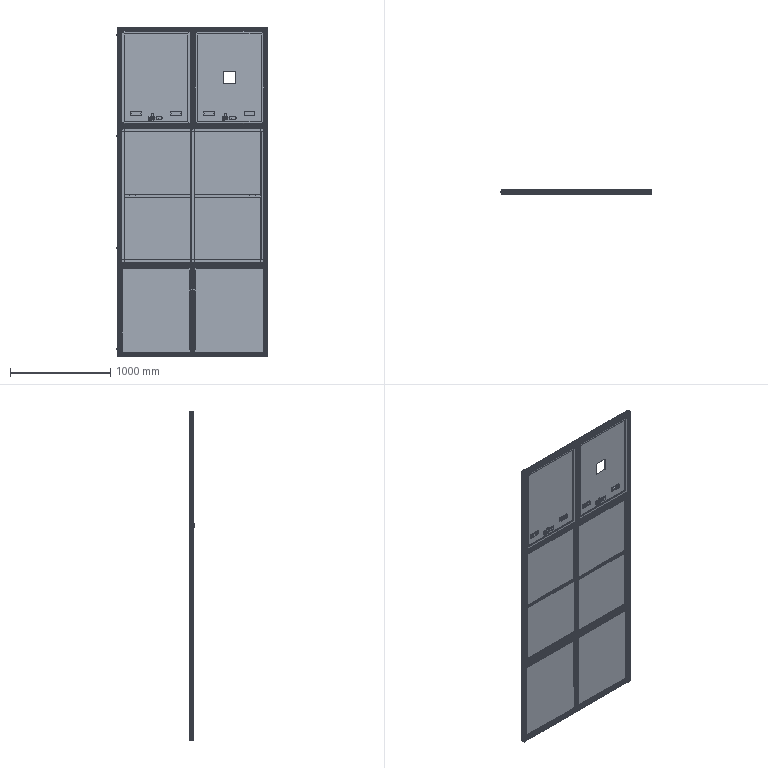Part | SolidWorks | 122 solids | 6208 faces | volume 28902679 mm3 | plane 3853 | cylinder 1823 | cone 314 | spline 206 | torus 12 | commonest cylinder face diameters 5 x224 6.8 x188 2 x182 1 x144 11 x136 8 x76